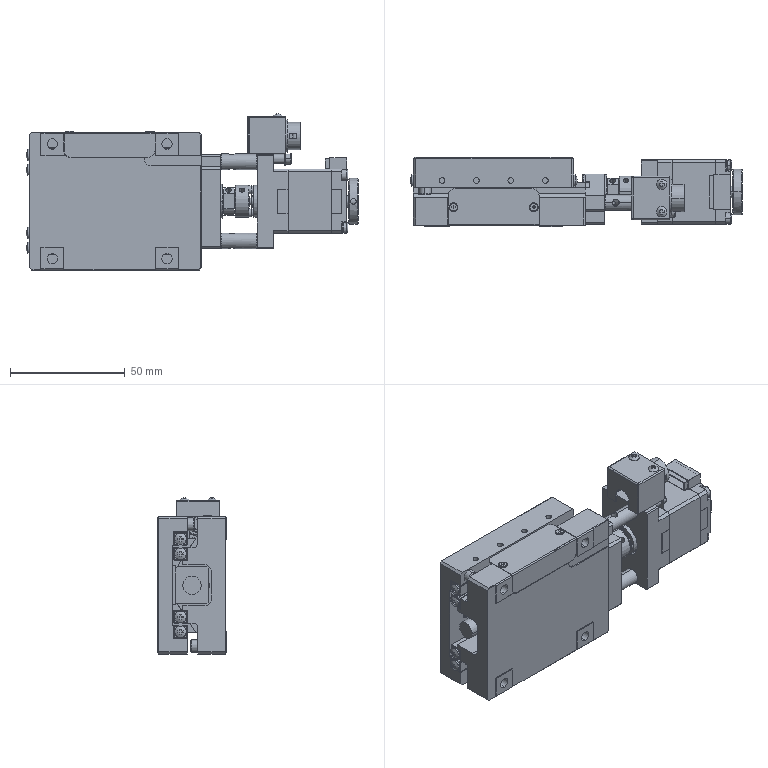Part | SolidWorks | 24 solids | 1949 faces | box 144.767 x 30 x 68.134 mm | volume 145224 mm3 | plane 1192 | cylinder 516 | cone 121 | torus 70 | spline 50 | commonest cylinder face diameters 4.5 x54 2.5 x50 5.5 x26 6 x25 0.6 x24 3.8 x20